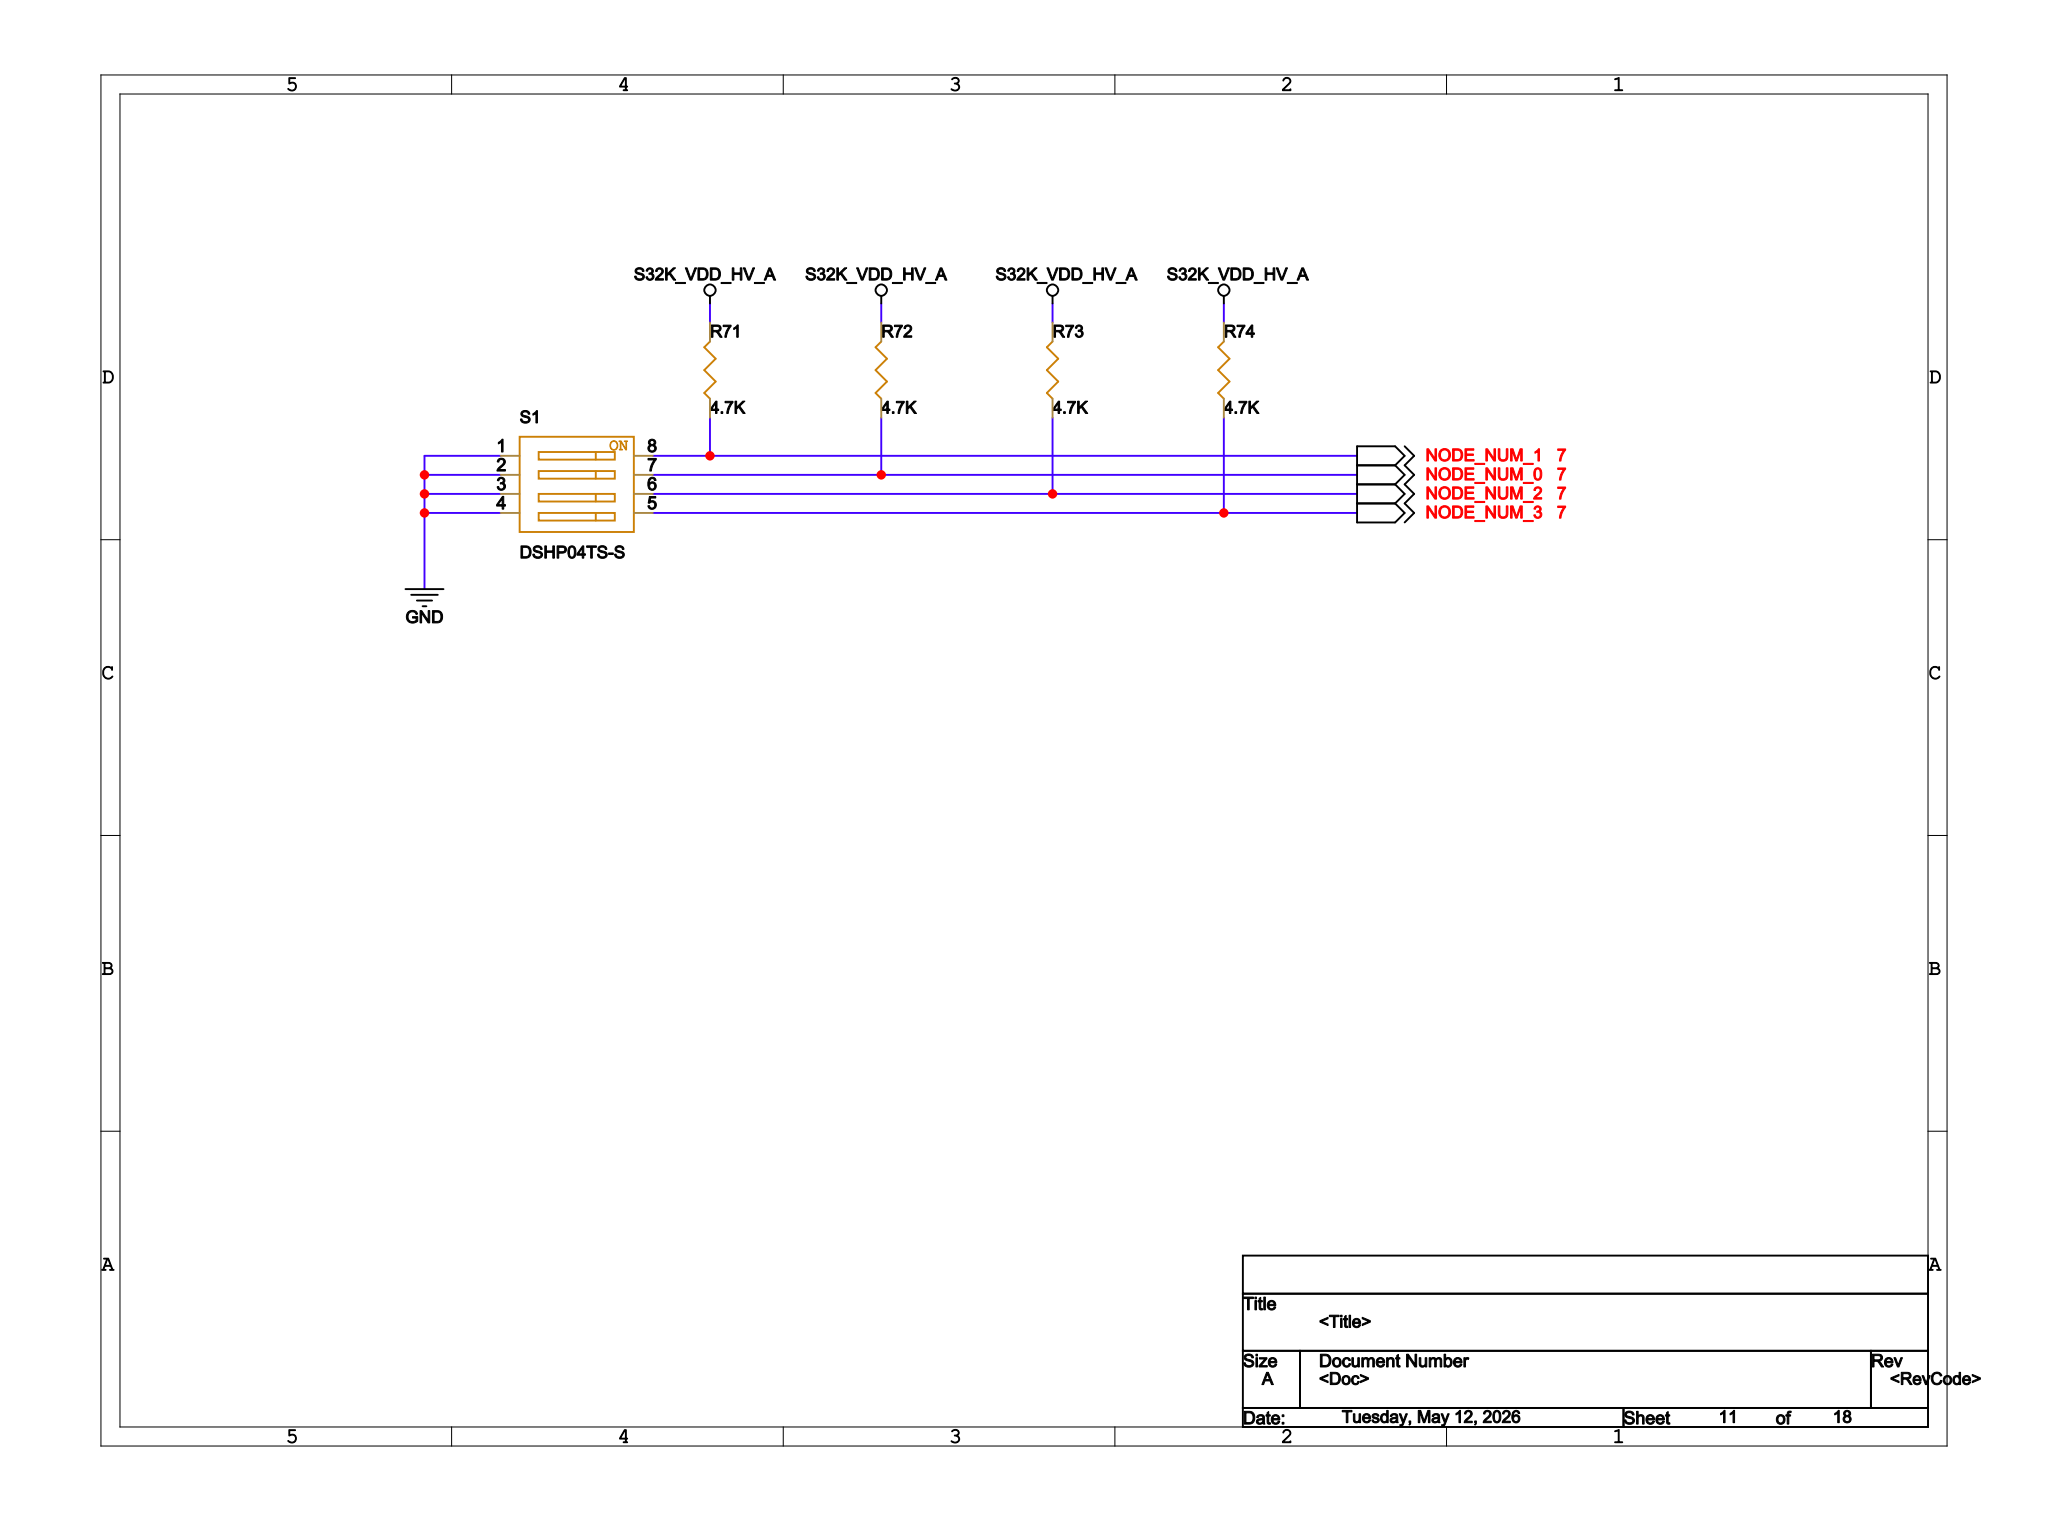Circuit board | Cadence Allegro | 330 parts | 215 nets | one sheet of the schematic
Parts on this sheet (reference | value | footprint):
R71 | 4.7K | 0402
R72 | 4.7K | 0402
R73 | 4.7K | 0402
R74 | 4.7K | 0402
S1 | DSHP04TS-S | DSHP04TS-S
Nets of these parts (net: part-pin ...):
GND: S1-1 S1-2 S1-3 S1-4
S32K_VDD_HV_A: R71-2 R72-2 R73-2 R74-2
NODE_NUM_1: R71-1 S1-8
NODE_NUM_0: R72-1 S1-7
NODE_NUM_2: R73-1 S1-6
NODE_NUM_3: R74-1 S1-5